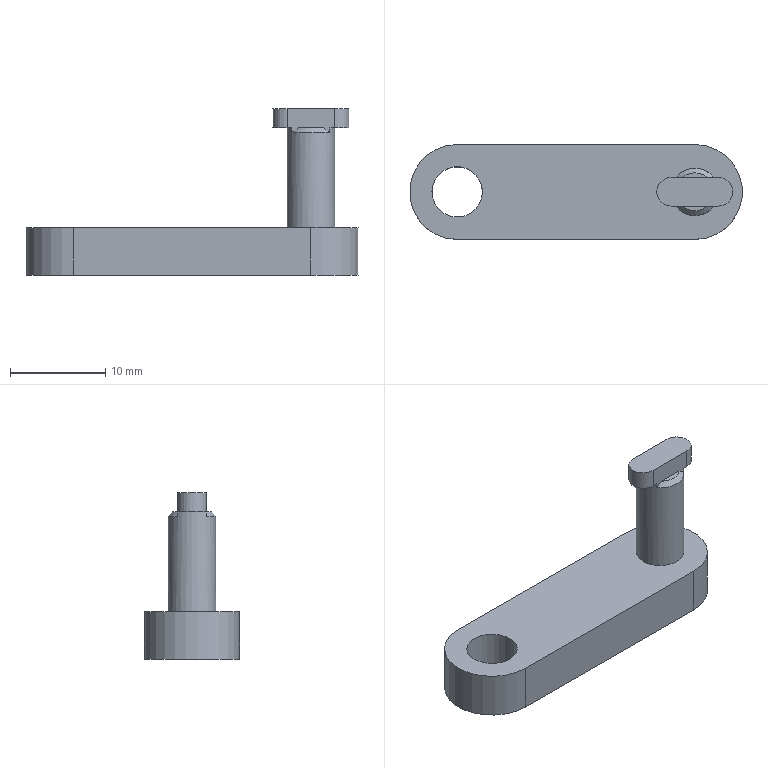Part | NX | features BREP 1 | 1 solid | 19 faces | box 35 x 10 x 17.5 mm | volume 1782 mm3 | plane 11 | cylinder 6 | cone 2 | commonest cylinder face diameters 3 x2 10 x2 5 x1 5.3 x1
STEP:
#1=CARTESIAN_POINT('',(10.,1.5,15.));
#2=VERTEX_POINT('',#1);
#3=CARTESIAN_POINT('',(10.,-1.5,15.));
#4=VERTEX_POINT('',#3);
#5=CARTESIAN_POINT('',(10.,0.,15.));
#6=DIRECTION('',(0.,0.,1.));
#7=DIRECTION('',(1.,0.,0.));
#8=AXIS2_PLACEMENT_3D('',#5,#6,#7);
#9=CIRCLE('',#8,1.5);
#10=EDGE_CURVE('',#2,#4,#9,.T.);
#11=ORIENTED_EDGE('',*,*,#10,.F.);
#12=CARTESIAN_POINT('',(10.,1.5,13.));
#13=VERTEX_POINT('',#12);
#14=CARTESIAN_POINT('',(10.,1.5,15.));
#15=DIRECTION('',(0.,0.,-1.));
#16=VECTOR('',#15,1000.);
#17=LINE('',#14,#16);
#18=EDGE_CURVE('',#2,#13,#17,.T.);
#19=ORIENTED_EDGE('',*,*,#18,.T.);
#20=CARTESIAN_POINT('',(10.,-1.5,13.));
#21=VERTEX_POINT('',#20);
#22=CARTESIAN_POINT('',(10.,0.,13.));
#23=DIRECTION('',(0.,0.,1.));
#24=DIRECTION('',(1.,0.,0.));
#25=AXIS2_PLACEMENT_3D('',#22,#23,#24);
#26=CIRCLE('',#25,1.5);
#27=EDGE_CURVE('',#13,#21,#26,.T.);
#28=ORIENTED_EDGE('',*,*,#27,.T.);
#29=CARTESIAN_POINT('',(10.,-1.5,15.));
#30=DIRECTION('',(0.,0.,-1.));
#31=VECTOR('',#30,1000.);
#32=LINE('',#29,#31);
#33=EDGE_CURVE('',#4,#21,#32,.T.);
#34=ORIENTED_EDGE('',*,*,#33,.F.);
#35=EDGE_LOOP('',(#11,#19,#28,#34));
#36=FACE_BOUND('',#35,.T.);
#37=CARTESIAN_POINT('',(10.,0.,15.));
#38=DIRECTION('',(0.,0.,-1.));
#39=DIRECTION('',(1.,0.,0.));
#40=AXIS2_PLACEMENT_3D('',#37,#38,#39);
#41=CYLINDRICAL_SURFACE('',#40,1.5);
#42=ADVANCED_FACE('',(#36),#41,.T.);
#43=CARTESIAN_POINT('',(15.,0.,2.5));
#44=VERTEX_POINT('',#43);
#45=CARTESIAN_POINT('',(12.5,0.,2.5));
#46=DIRECTION('',(0.,0.,1.));
#47=DIRECTION('',(1.,0.,0.));
#48=AXIS2_PLACEMENT_3D('',#45,#46,#47);
#49=CIRCLE('',#48,2.5);
#50=EDGE_CURVE('',#44,#44,#49,.T.);
#51=ORIENTED_EDGE('',*,*,#50,.T.);
#52=EDGE_LOOP('',(#51));
#53=FACE_BOUND('',#52,.T.);
#54=CARTESIAN_POINT('',(14.5,-1.5,13.));
#55=VERTEX_POINT('',#54);
#56=CARTESIAN_POINT('',(14.5,1.5,13.));
#57=VERTEX_POINT('',#56);
#58=CARTESIAN_POINT('',(12.5,0.,13.));
#59=DIRECTION('',(0.,0.,1.));
#60=DIRECTION('',(1.,0.,0.));
#61=AXIS2_PLACEMENT_3D('',#58,#59,#60);
#62=CIRCLE('',#61,2.5);
#63=EDGE_CURVE('',#55,#57,#62,.T.);
#64=ORIENTED_EDGE('',*,*,#63,.F.);
#65=CARTESIAN_POINT('',(14.5,-1.5,12.5));
#66=VERTEX_POINT('',#65);
#67=CARTESIAN_POINT('',(14.5,-1.5,13.));
#68=DIRECTION('',(0.,0.,-1.));
#69=VECTOR('',#68,1000.);
#70=LINE('',#67,#69);
#71=EDGE_CURVE('',#55,#66,#70,.T.);
#72=ORIENTED_EDGE('',*,*,#71,.T.);
#73=CARTESIAN_POINT('',(10.5,-1.5,12.5));
#74=VERTEX_POINT('',#73);
#75=CARTESIAN_POINT('',(12.5,0.,12.5));
#76=DIRECTION('',(0.,0.,-1.));
#77=DIRECTION('',(1.,0.,0.));
#78=AXIS2_PLACEMENT_3D('',#75,#76,#77);
#79=CIRCLE('',#78,2.5);
#80=EDGE_CURVE('',#66,#74,#79,.T.);
#81=ORIENTED_EDGE('',*,*,#80,.T.);
#82=CARTESIAN_POINT('',(10.5,-1.5,13.));
#83=VERTEX_POINT('',#82);
#84=CARTESIAN_POINT('',(10.5,-1.5,12.5));
#85=DIRECTION('',(0.,0.,1.));
#86=VECTOR('',#85,1000.);
#87=LINE('',#84,#86);
#88=EDGE_CURVE('',#74,#83,#87,.T.);
#89=ORIENTED_EDGE('',*,*,#88,.T.);
#90=CARTESIAN_POINT('',(10.5,1.5,13.));
#91=VERTEX_POINT('',#90);
#92=CARTESIAN_POINT('',(12.5,0.,13.));
#93=DIRECTION('',(0.,0.,1.));
#94=DIRECTION('',(1.,0.,0.));
#95=AXIS2_PLACEMENT_3D('',#92,#93,#94);
#96=CIRCLE('',#95,2.5);
#97=EDGE_CURVE('',#91,#83,#96,.T.);
#98=ORIENTED_EDGE('',*,*,#97,.F.);
#99=CARTESIAN_POINT('',(10.5,1.5,12.5));
#100=VERTEX_POINT('',#99);
#101=CARTESIAN_POINT('',(10.5,1.5,13.));
#102=DIRECTION('',(0.,0.,-1.));
#103=VECTOR('',#102,1000.);
#104=LINE('',#101,#103);
#105=EDGE_CURVE('',#91,#100,#104,.T.);
#106=ORIENTED_EDGE('',*,*,#105,.T.);
#107=CARTESIAN_POINT('',(14.5,1.5,12.5));
#108=VERTEX_POINT('',#107);
#109=CARTESIAN_POINT('',(12.5,0.,12.5));
#110=DIRECTION('',(0.,0.,-1.));
#111=DIRECTION('',(1.,0.,0.));
#112=AXIS2_PLACEMENT_3D('',#109,#110,#111);
#113=CIRCLE('',#112,2.5);
#114=EDGE_CURVE('',#100,#108,#113,.T.);
#115=ORIENTED_EDGE('',*,*,#114,.T.);
#116=CARTESIAN_POINT('',(14.5,1.5,12.5));
#117=DIRECTION('',(0.,0.,1.));
#118=VECTOR('',#117,1000.);
#119=LINE('',#116,#118);
#120=EDGE_CURVE('',#108,#57,#119,.T.);
#121=ORIENTED_EDGE('',*,*,#120,.T.);
#122=EDGE_LOOP('',(#64,#72,#81,#89,#98,#106,#115,#121));
#123=FACE_BOUND('',#122,.T.);
#124=CARTESIAN_POINT('',(12.5,0.,7.7));
#125=DIRECTION('',(0.,0.,-1.));
#126=DIRECTION('',(1.,0.,0.));
#127=AXIS2_PLACEMENT_3D('',#124,#125,#126);
#128=CYLINDRICAL_SURFACE('',#127,2.5);
#129=ADVANCED_FACE('',(#53,#123),#128,.T.);
#130=CARTESIAN_POINT('',(-9.85,0.,-2.5));
#131=VERTEX_POINT('',#130);
#132=CARTESIAN_POINT('',(-12.5,0.,-2.5));
#133=DIRECTION('',(0.,0.,1.));
#134=DIRECTION('',(1.,0.,0.));
#135=AXIS2_PLACEMENT_3D('',#132,#133,#134);
#136=CIRCLE('',#135,2.65);
#137=EDGE_CURVE('',#131,#131,#136,.T.);
#138=ORIENTED_EDGE('',*,*,#137,.F.);
#139=EDGE_LOOP('',(#138));
#140=FACE_BOUND('',#139,.T.);
#141=CARTESIAN_POINT('',(-9.85,0.,2.5));
#142=VERTEX_POINT('',#141);
#143=CARTESIAN_POINT('',(-12.5,0.,2.5));
#144=DIRECTION('',(0.,0.,1.));
#145=DIRECTION('',(1.,0.,0.));
#146=AXIS2_PLACEMENT_3D('',#143,#144,#145);
#147=CIRCLE('',#146,2.65);
#148=EDGE_CURVE('',#142,#142,#147,.T.);
#149=ORIENTED_EDGE('',*,*,#148,.T.);
#150=EDGE_LOOP('',(#149));
#151=FACE_BOUND('',#150,.T.);
#152=CARTESIAN_POINT('',(-12.5,0.,2.5));
#153=DIRECTION('',(0.,0.,-1.));
#154=DIRECTION('',(1.,0.,0.));
#155=AXIS2_PLACEMENT_3D('',#152,#153,#154);
#156=CYLINDRICAL_SURFACE('',#155,2.65);
#157=ADVANCED_FACE('',(#140,#151),#156,.F.);
#158=CARTESIAN_POINT('',(-12.5,5.,2.5));
#159=VERTEX_POINT('',#158);
#160=CARTESIAN_POINT('',(-12.5,-5.,2.5));
#161=VERTEX_POINT('',#160);
#162=CARTESIAN_POINT('',(-12.5,0.,2.5));
#163=DIRECTION('',(0.,0.,1.));
#164=DIRECTION('',(1.,0.,0.));
#165=AXIS2_PLACEMENT_3D('',#162,#163,#164);
#166=CIRCLE('',#165,5.);
#167=EDGE_CURVE('',#159,#161,#166,.T.);
#168=ORIENTED_EDGE('',*,*,#167,.F.);
#169=CARTESIAN_POINT('',(-12.5,5.,-2.5));
#170=VERTEX_POINT('',#169);
#171=CARTESIAN_POINT('',(-12.5,5.,2.5));
#172=DIRECTION('',(0.,0.,-1.));
#173=VECTOR('',#172,1000.);
#174=LINE('',#171,#173);
#175=EDGE_CURVE('',#159,#170,#174,.T.);
#176=ORIENTED_EDGE('',*,*,#175,.T.);
#177=CARTESIAN_POINT('',(-12.5,-5.,-2.5));
#178=VERTEX_POINT('',#177);
#179=CARTESIAN_POINT('',(-12.5,0.,-2.5));
#180=DIRECTION('',(0.,0.,1.));
#181=DIRECTION('',(1.,0.,0.));
#182=AXIS2_PLACEMENT_3D('',#179,#180,#181);
#183=CIRCLE('',#182,5.);
#184=EDGE_CURVE('',#170,#178,#183,.T.);
#185=ORIENTED_EDGE('',*,*,#184,.T.);
#186=CARTESIAN_POINT('',(-12.5,-5.,2.5));
#187=DIRECTION('',(0.,0.,-1.));
#188=VECTOR('',#187,1000.);
#189=LINE('',#186,#188);
#190=EDGE_CURVE('',#161,#178,#189,.T.);
#191=ORIENTED_EDGE('',*,*,#190,.F.);
#192=EDGE_LOOP('',(#168,#176,#185,#191));
#193=FACE_BOUND('',#192,.T.);
#194=CARTESIAN_POINT('',(-12.5,0.,2.5));
#195=DIRECTION('',(0.,0.,-1.));
#196=DIRECTION('',(1.,0.,0.));
#197=AXIS2_PLACEMENT_3D('',#194,#195,#196);
#198=CYLINDRICAL_SURFACE('',#197,5.);
#199=ADVANCED_FACE('',(#193),#198,.T.);
#200=CARTESIAN_POINT('',(13.823,1.5,13.));
#201=VERTEX_POINT('',#200);
#202=CARTESIAN_POINT('',(11.177,1.5,13.));
#203=VERTEX_POINT('',#202);
#204=CARTESIAN_POINT('',(10.,1.5,13.));
#205=DIRECTION('',(-1.,0.,0.));
#206=VECTOR('',#205,1000.);
#207=LINE('',#204,#206);
#208=EDGE_CURVE('',#201,#203,#207,.T.);
#209=ORIENTED_EDGE('',*,*,#208,.F.);
#210=CARTESIAN_POINT('',(12.5,0.,13.));
#211=DIRECTION('',(0.,0.,1.));
#212=DIRECTION('',(1.,0.,0.));
#213=AXIS2_PLACEMENT_3D('',#210,#211,#212);
#214=CIRCLE('',#213,2.);
#215=EDGE_CURVE('',#201,#203,#214,.T.);
#216=ORIENTED_EDGE('',*,*,#215,.T.);
#217=EDGE_LOOP('',(#209,#216));
#218=FACE_BOUND('',#217,.T.);
#219=CARTESIAN_POINT('',(12.5,0.,13.));
#220=DIRECTION('',(0.,0.,1.));
#221=DIRECTION('',(-1.,0.,0.));
#222=AXIS2_PLACEMENT_3D('',#219,#220,#221);
#223=PLANE('',#222);
#224=ADVANCED_FACE('',(#218),#223,.T.);
#225=ORIENTED_EDGE('',*,*,#148,.F.);
#226=EDGE_LOOP('',(#225));
#227=FACE_BOUND('',#226,.T.);
#228=CARTESIAN_POINT('',(12.5,5.,2.5));
#229=VERTEX_POINT('',#228);
#230=CARTESIAN_POINT('',(-12.5,5.,2.5));
#231=DIRECTION('',(-1.,0.,0.));
#232=VECTOR('',#231,1000.);
#233=LINE('',#230,#232);
#234=EDGE_CURVE('',#229,#159,#233,.T.);
#235=ORIENTED_EDGE('',*,*,#234,.T.);
#236=ORIENTED_EDGE('',*,*,#167,.T.);
#237=CARTESIAN_POINT('',(12.5,-5.,2.5));
#238=VERTEX_POINT('',#237);
#239=CARTESIAN_POINT('',(-12.5,-5.,2.5));
#240=DIRECTION('',(1.,0.,0.));
#241=VECTOR('',#240,1000.);
#242=LINE('',#239,#241);
#243=EDGE_CURVE('',#161,#238,#242,.T.);
#244=ORIENTED_EDGE('',*,*,#243,.T.);
#245=CARTESIAN_POINT('',(12.5,0.,2.5));
#246=DIRECTION('',(0.,0.,1.));
#247=DIRECTION('',(1.,0.,0.));
#248=AXIS2_PLACEMENT_3D('',#245,#246,#247);
#249=CIRCLE('',#248,5.);
#250=EDGE_CURVE('',#238,#229,#249,.T.);
#251=ORIENTED_EDGE('',*,*,#250,.T.);
#252=EDGE_LOOP('',(#235,#236,#244,#251));
#253=FACE_BOUND('',#252,.T.);
#254=ORIENTED_EDGE('',*,*,#50,.F.);
#255=EDGE_LOOP('',(#254));
#256=FACE_BOUND('',#255,.T.);
#257=CARTESIAN_POINT('',(-12.5,0.,2.5));
#258=DIRECTION('',(0.,0.,1.));
#259=DIRECTION('',(-1.,0.,0.));
#260=AXIS2_PLACEMENT_3D('',#257,#258,#259);
#261=PLANE('',#260);
#262=ADVANCED_FACE('',(#227,#253,#256),#261,.T.);
#263=ORIENTED_EDGE('',*,*,#184,.F.);
#264=CARTESIAN_POINT('',(12.5,5.,-2.5));
#265=VERTEX_POINT('',#264);
#266=CARTESIAN_POINT('',(-12.5,5.,-2.5));
#267=DIRECTION('',(-1.,0.,0.));
#268=VECTOR('',#267,1000.);
#269=LINE('',#266,#268);
#270=EDGE_CURVE('',#265,#170,#269,.T.);
#271=ORIENTED_EDGE('',*,*,#270,.F.);
#272=CARTESIAN_POINT('',(12.5,-5.,-2.5));
#273=VERTEX_POINT('',#272);
#274=CARTESIAN_POINT('',(12.5,0.,-2.5));
#275=DIRECTION('',(0.,0.,1.));
#276=DIRECTION('',(1.,0.,0.));
#277=AXIS2_PLACEMENT_3D('',#274,#275,#276);
#278=CIRCLE('',#277,5.);
#279=EDGE_CURVE('',#273,#265,#278,.T.);
#280=ORIENTED_EDGE('',*,*,#279,.F.);
#281=CARTESIAN_POINT('',(-12.5,-5.,-2.5));
#282=DIRECTION('',(1.,0.,0.));
#283=VECTOR('',#282,1000.);
#284=LINE('',#281,#283);
#285=EDGE_CURVE('',#178,#273,#284,.T.);
#286=ORIENTED_EDGE('',*,*,#285,.F.);
#287=EDGE_LOOP('',(#263,#271,#280,#286));
#288=FACE_BOUND('',#287,.T.);
#289=ORIENTED_EDGE('',*,*,#137,.T.);
#290=EDGE_LOOP('',(#289));
#291=FACE_BOUND('',#290,.T.);
#292=CARTESIAN_POINT('',(-12.5,0.,-2.5));
#293=DIRECTION('',(0.,0.,1.));
#294=DIRECTION('',(-1.,0.,0.));
#295=AXIS2_PLACEMENT_3D('',#292,#293,#294);
#296=PLANE('',#295);
#297=ADVANCED_FACE('',(#288,#291),#296,.F.);
#298=ORIENTED_EDGE('',*,*,#285,.T.);
#299=CARTESIAN_POINT('',(12.5,-5.,2.5));
#300=DIRECTION('',(0.,0.,-1.));
#301=VECTOR('',#300,1000.);
#302=LINE('',#299,#301);
#303=EDGE_CURVE('',#238,#273,#302,.T.);
#304=ORIENTED_EDGE('',*,*,#303,.F.);
#305=ORIENTED_EDGE('',*,*,#243,.F.);
#306=ORIENTED_EDGE('',*,*,#190,.T.);
#307=EDGE_LOOP('',(#298,#304,#305,#306));
#308=FACE_BOUND('',#307,.T.);
#309=CARTESIAN_POINT('',(-12.5,-5.,2.5));
#310=DIRECTION('',(0.,1.,0.));
#311=DIRECTION('',(0.,0.,-1.));
#312=AXIS2_PLACEMENT_3D('',#309,#310,#311);
#313=PLANE('',#312);
#314=ADVANCED_FACE('',(#308),#313,.F.);
#315=ORIENTED_EDGE('',*,*,#279,.T.);
#316=CARTESIAN_POINT('',(12.5,5.,2.5));
#317=DIRECTION('',(0.,0.,-1.));
#318=VECTOR('',#317,1000.);
#319=LINE('',#316,#318);
#320=EDGE_CURVE('',#229,#265,#319,.T.);
#321=ORIENTED_EDGE('',*,*,#320,.F.);
#322=ORIENTED_EDGE('',*,*,#250,.F.);
#323=ORIENTED_EDGE('',*,*,#303,.T.);
#324=EDGE_LOOP('',(#315,#321,#322,#323));
#325=FACE_BOUND('',#324,.T.);
#326=CARTESIAN_POINT('',(12.5,0.,2.5));
#327=DIRECTION('',(0.,0.,-1.));
#328=DIRECTION('',(1.,0.,0.));
#329=AXIS2_PLACEMENT_3D('',#326,#327,#328);
#330=CYLINDRICAL_SURFACE('',#329,5.);
#331=ADVANCED_FACE('',(#325),#330,.T.);
#332=ORIENTED_EDGE('',*,*,#270,.T.);
#333=ORIENTED_EDGE('',*,*,#175,.F.);
#334=ORIENTED_EDGE('',*,*,#234,.F.);
#335=ORIENTED_EDGE('',*,*,#320,.T.);
#336=EDGE_LOOP('',(#332,#333,#334,#335));
#337=FACE_BOUND('',#336,.T.);
#338=CARTESIAN_POINT('',(-12.5,5.,2.5));
#339=DIRECTION('',(0.,-1.,0.));
#340=DIRECTION('',(-1.,0.,0.));
#341=AXIS2_PLACEMENT_3D('',#338,#339,#340);
#342=PLANE('',#341);
#343=ADVANCED_FACE('',(#337),#342,.F.);
#344=CARTESIAN_POINT('',(11.177,-1.5,13.));
#345=VERTEX_POINT('',#344);
#346=CARTESIAN_POINT('',(13.823,-1.5,13.));
#347=VERTEX_POINT('',#346);
#348=CARTESIAN_POINT('',(10.,-1.5,13.));
#349=DIRECTION('',(1.,0.,0.));
#350=VECTOR('',#349,1000.);
#351=LINE('',#348,#350);
#352=EDGE_CURVE('',#345,#347,#351,.T.);
#353=ORIENTED_EDGE('',*,*,#352,.F.);
#354=CARTESIAN_POINT('',(12.5,0.,13.));
#355=DIRECTION('',(0.,0.,1.));
#356=DIRECTION('',(1.,0.,0.));
#357=AXIS2_PLACEMENT_3D('',#354,#355,#356);
#358=CIRCLE('',#357,2.);
#359=EDGE_CURVE('',#345,#347,#358,.T.);
#360=ORIENTED_EDGE('',*,*,#359,.T.);
#361=EDGE_LOOP('',(#353,#360));
#362=FACE_BOUND('',#361,.T.);
#363=CARTESIAN_POINT('',(12.5,0.,13.));
#364=DIRECTION('',(0.,0.,1.));
#365=DIRECTION('',(-1.,0.,0.));
#366=AXIS2_PLACEMENT_3D('',#363,#364,#365);
#367=PLANE('',#366);
#368=ADVANCED_FACE('',(#362),#367,.T.);
#369=CARTESIAN_POINT('',(10.,1.5,13.));
#370=DIRECTION('',(-1.,0.,0.));
#371=VECTOR('',#370,1000.);
#372=LINE('',#369,#371);
#373=EDGE_CURVE('',#91,#13,#372,.T.);
#374=ORIENTED_EDGE('',*,*,#373,.F.);
#375=ORIENTED_EDGE('',*,*,#97,.T.);
#376=CARTESIAN_POINT('',(10.,-1.5,13.));
#377=DIRECTION('',(1.,0.,0.));
#378=VECTOR('',#377,1000.);
#379=LINE('',#376,#378);
#380=EDGE_CURVE('',#21,#83,#379,.T.);
#381=ORIENTED_EDGE('',*,*,#380,.F.);
#382=ORIENTED_EDGE('',*,*,#27,.F.);
#383=EDGE_LOOP('',(#374,#375,#381,#382));
#384=FACE_BOUND('',#383,.T.);
#385=CARTESIAN_POINT('',(10.,0.,13.));
#386=DIRECTION('',(0.,0.,1.));
#387=DIRECTION('',(-1.,0.,0.));
#388=AXIS2_PLACEMENT_3D('',#385,#386,#387);
#389=PLANE('',#388);
#390=ADVANCED_FACE('',(#384),#389,.F.);
#391=CARTESIAN_POINT('',(15.,-1.5,13.));
#392=VERTEX_POINT('',#391);
#393=CARTESIAN_POINT('',(10.,-1.5,13.));
#394=DIRECTION('',(1.,0.,0.));
#395=VECTOR('',#394,1000.);
#396=LINE('',#393,#395);
#397=EDGE_CURVE('',#55,#392,#396,.T.);
#398=ORIENTED_EDGE('',*,*,#397,.F.);
#399=ORIENTED_EDGE('',*,*,#63,.T.);
#400=CARTESIAN_POINT('',(15.,1.5,13.));
#401=VERTEX_POINT('',#400);
#402=CARTESIAN_POINT('',(10.,1.5,13.));
#403=DIRECTION('',(-1.,0.,0.));
#404=VECTOR('',#403,1000.);
#405=LINE('',#402,#404);
#406=EDGE_CURVE('',#401,#57,#405,.T.);
#407=ORIENTED_EDGE('',*,*,#406,.F.);
#408=CARTESIAN_POINT('',(15.,0.,13.));
#409=DIRECTION('',(0.,0.,1.));
#410=DIRECTION('',(1.,0.,0.));
#411=AXIS2_PLACEMENT_3D('',#408,#409,#410);
#412=CIRCLE('',#411,1.5);
#413=EDGE_CURVE('',#392,#401,#412,.T.);
#414=ORIENTED_EDGE('',*,*,#413,.F.);
#415=EDGE_LOOP('',(#398,#399,#407,#414));
#416=FACE_BOUND('',#415,.T.);
#417=CARTESIAN_POINT('',(10.,0.,13.));
#418=DIRECTION('',(0.,0.,1.));
#419=DIRECTION('',(-1.,0.,0.));
#420=AXIS2_PLACEMENT_3D('',#417,#418,#419);
#421=PLANE('',#420);
#422=ADVANCED_FACE('',(#416),#421,.F.);
#423=ORIENTED_EDGE('',*,*,#380,.T.);
#424=ORIENTED_EDGE('',*,*,#88,.F.);
#425=CARTESIAN_POINT('',(10.5,-1.5,12.5));
#426=CARTESIAN_POINT('',(10.719,-1.5,12.675));
#427=CARTESIAN_POINT('',(10.943,-1.5,12.845));
#428=CARTESIAN_POINT('',(11.177,-1.5,13.));
#429=B_SPLINE_CURVE_WITH_KNOTS('',3,(#425,#426,#427,#428),.UNSPECIFIED.,.F.,.F.,(4,4),(0.,0.0008417),.UNSPECIFIED.);
#430=EDGE_CURVE('',#74,#345,#429,.T.);
#431=ORIENTED_EDGE('',*,*,#430,.T.);
#432=ORIENTED_EDGE('',*,*,#352,.T.);
#433=CARTESIAN_POINT('',(13.823,-1.5,13.));
#434=CARTESIAN_POINT('',(14.057,-1.5,12.845));
#435=CARTESIAN_POINT('',(14.281,-1.5,12.675));
#436=CARTESIAN_POINT('',(14.5,-1.5,12.5));
#437=B_SPLINE_CURVE_WITH_KNOTS('',3,(#433,#434,#435,#436),.UNSPECIFIED.,.F.,.F.,(4,4),(0.,0.0008417),.UNSPECIFIED.);
#438=EDGE_CURVE('',#347,#66,#437,.T.);
#439=ORIENTED_EDGE('',*,*,#438,.T.);
#440=ORIENTED_EDGE('',*,*,#71,.F.);
#441=ORIENTED_EDGE('',*,*,#397,.T.);
#442=CARTESIAN_POINT('',(15.,-1.5,15.));
#443=VERTEX_POINT('',#442);
#444=CARTESIAN_POINT('',(15.,-1.5,15.));
#445=DIRECTION('',(0.,0.,-1.));
#446=VECTOR('',#445,1000.);
#447=LINE('',#444,#446);
#448=EDGE_CURVE('',#443,#392,#447,.T.);
#449=ORIENTED_EDGE('',*,*,#448,.F.);
#450=CARTESIAN_POINT('',(10.,-1.5,15.));
#451=DIRECTION('',(1.,0.,0.));
#452=VECTOR('',#451,1000.);
#453=LINE('',#450,#452);
#454=EDGE_CURVE('',#4,#443,#453,.T.);
#455=ORIENTED_EDGE('',*,*,#454,.F.);
#456=ORIENTED_EDGE('',*,*,#33,.T.);
#457=EDGE_LOOP('',(#423,#424,#431,#432,#439,#440,#441,#449,#455,#456));
#458=FACE_BOUND('',#457,.T.);
#459=CARTESIAN_POINT('',(10.,-1.5,15.));
#460=DIRECTION('',(0.,1.,0.));
#461=DIRECTION('',(0.,0.,-1.));
#462=AXIS2_PLACEMENT_3D('',#459,#460,#461);
#463=PLANE('',#462);
#464=ADVANCED_FACE('',(#458),#463,.F.);
#465=ORIENTED_EDGE('',*,*,#413,.T.);
#466=CARTESIAN_POINT('',(15.,1.5,15.));
#467=VERTEX_POINT('',#466);
#468=CARTESIAN_POINT('',(15.,1.5,15.));
#469=DIRECTION('',(0.,0.,-1.));
#470=VECTOR('',#469,1000.);
#471=LINE('',#468,#470);
#472=EDGE_CURVE('',#467,#401,#471,.T.);
#473=ORIENTED_EDGE('',*,*,#472,.F.);
#474=CARTESIAN_POINT('',(15.,0.,15.));
#475=DIRECTION('',(0.,0.,1.));
#476=DIRECTION('',(1.,0.,0.));
#477=AXIS2_PLACEMENT_3D('',#474,#475,#476);
#478=CIRCLE('',#477,1.5);
#479=EDGE_CURVE('',#443,#467,#478,.T.);
#480=ORIENTED_EDGE('',*,*,#479,.F.);
#481=ORIENTED_EDGE('',*,*,#448,.T.);
#482=EDGE_LOOP('',(#465,#473,#480,#481));
#483=FACE_BOUND('',#482,.T.);
#484=CARTESIAN_POINT('',(15.,0.,15.));
#485=DIRECTION('',(0.,0.,-1.));
#486=DIRECTION('',(1.,0.,0.));
#487=AXIS2_PLACEMENT_3D('',#484,#485,#486);
#488=CYLINDRICAL_SURFACE('',#487,1.5);
#489=ADVANCED_FACE('',(#483),#488,.T.);
#490=ORIENTED_EDGE('',*,*,#406,.T.);
#491=ORIENTED_EDGE('',*,*,#120,.F.);
#492=CARTESIAN_POINT('',(14.5,1.5,12.5));
#493=CARTESIAN_POINT('',(14.281,1.5,12.675));
#494=CARTESIAN_POINT('',(14.057,1.5,12.845));
#495=CARTESIAN_POINT('',(13.823,1.5,13.));
#496=B_SPLINE_CURVE_WITH_KNOTS('',3,(#492,#493,#494,#495),.UNSPECIFIED.,.F.,.F.,(4,4),(0.,0.0008417),.UNSPECIFIED.);
#497=EDGE_CURVE('',#108,#201,#496,.T.);
#498=ORIENTED_EDGE('',*,*,#497,.T.);
#499=ORIENTED_EDGE('',*,*,#208,.T.);
#500=CARTESIAN_POINT('',(11.177,1.5,13.));
#501=CARTESIAN_POINT('',(10.943,1.5,12.845));
#502=CARTESIAN_POINT('',(10.719,1.5,12.675));
#503=CARTESIAN_POINT('',(10.5,1.5,12.5));
#504=B_SPLINE_CURVE_WITH_KNOTS('',3,(#500,#501,#502,#503),.UNSPECIFIED.,.F.,.F.,(4,4),(0.,0.0008417),.UNSPECIFIED.);
#505=EDGE_CURVE('',#203,#100,#504,.T.);
#506=ORIENTED_EDGE('',*,*,#505,.T.);
#507=ORIENTED_EDGE('',*,*,#105,.F.);
#508=ORIENTED_EDGE('',*,*,#373,.T.);
#509=ORIENTED_EDGE('',*,*,#18,.F.);
#510=CARTESIAN_POINT('',(10.,1.5,15.));
#511=DIRECTION('',(-1.,0.,0.));
#512=VECTOR('',#511,1000.);
#513=LINE('',#510,#512);
#514=EDGE_CURVE('',#467,#2,#513,.T.);
#515=ORIENTED_EDGE('',*,*,#514,.F.);
#516=ORIENTED_EDGE('',*,*,#472,.T.);
#517=EDGE_LOOP('',(#490,#491,#498,#499,#506,#507,#508,#509,#515,#516));
#518=FACE_BOUND('',#517,.T.);
#519=CARTESIAN_POINT('',(10.,1.5,15.));
#520=DIRECTION('',(0.,-1.,0.));
#521=DIRECTION('',(0.,0.,1.));
#522=AXIS2_PLACEMENT_3D('',#519,#520,#521);
#523=PLANE('',#522);
#524=ADVANCED_FACE('',(#518),#523,.F.);
#525=ORIENTED_EDGE('',*,*,#514,.T.);
#526=ORIENTED_EDGE('',*,*,#10,.T.);
#527=ORIENTED_EDGE('',*,*,#454,.T.);
#528=ORIENTED_EDGE('',*,*,#479,.T.);
#529=EDGE_LOOP('',(#525,#526,#527,#528));
#530=FACE_BOUND('',#529,.T.);
#531=CARTESIAN_POINT('',(10.,0.,15.));
#532=DIRECTION('',(0.,0.,1.));
#533=DIRECTION('',(-1.,0.,0.));
#534=AXIS2_PLACEMENT_3D('',#531,#532,#533);
#535=PLANE('',#534);
#536=ADVANCED_FACE('',(#530),#535,.T.);
#537=ORIENTED_EDGE('',*,*,#430,.F.);
#538=ORIENTED_EDGE('',*,*,#80,.F.);
#539=ORIENTED_EDGE('',*,*,#438,.F.);
#540=ORIENTED_EDGE('',*,*,#359,.F.);
#541=EDGE_LOOP('',(#537,#538,#539,#540));
#542=FACE_BOUND('',#541,.T.);
#543=CARTESIAN_POINT('',(12.5,0.,13.));
#544=DIRECTION('',(0.,0.,-1.));
#545=DIRECTION('',(1.,0.,0.));
#546=AXIS2_PLACEMENT_3D('',#543,#544,#545);
#547=CONICAL_SURFACE('',#546,2.,0.7854);
#548=ADVANCED_FACE('',(#542),#547,.T.);
#549=ORIENTED_EDGE('',*,*,#497,.F.);
#550=ORIENTED_EDGE('',*,*,#114,.F.);
#551=ORIENTED_EDGE('',*,*,#505,.F.);
#552=ORIENTED_EDGE('',*,*,#215,.F.);
#553=EDGE_LOOP('',(#549,#550,#551,#552));
#554=FACE_BOUND('',#553,.T.);
#555=CARTESIAN_POINT('',(12.5,0.,13.));
#556=DIRECTION('',(0.,0.,-1.));
#557=DIRECTION('',(1.,0.,0.));
#558=AXIS2_PLACEMENT_3D('',#555,#556,#557);
#559=CONICAL_SURFACE('',#558,2.,0.7854);
#560=ADVANCED_FACE('',(#554),#559,.T.);
#561=CLOSED_SHELL('',(#42,#129,#157,#199,#224,#262,#297,#314,#331,#343,#368,#390,#422,#464,#489,#524,#536,#548,#560));
#562=MANIFOLD_SOLID_BREP('',#561);
#563=(LENGTH_UNIT()NAMED_UNIT(*)SI_UNIT(.MILLI.,.METRE.));
#564=UNCERTAINTY_MEASURE_WITH_UNIT(LENGTH_MEASURE(0.0508),#563,'','');
#565=(NAMED_UNIT(*)PLANE_ANGLE_UNIT()SI_UNIT($,.RADIAN.));
#566=(NAMED_UNIT(*)SI_UNIT($,.STERADIAN.)SOLID_ANGLE_UNIT());
#567=(GEOMETRIC_REPRESENTATION_CONTEXT(3)GLOBAL_UNCERTAINTY_ASSIGNED_CONTEXT((#564))GLOBAL_UNIT_ASSIGNED_CONTEXT((#563,#565,#566))REPRESENTATION_CONTEXT('',''));
#568=ADVANCED_BREP_SHAPE_REPRESENTATION('',(#562),#567);